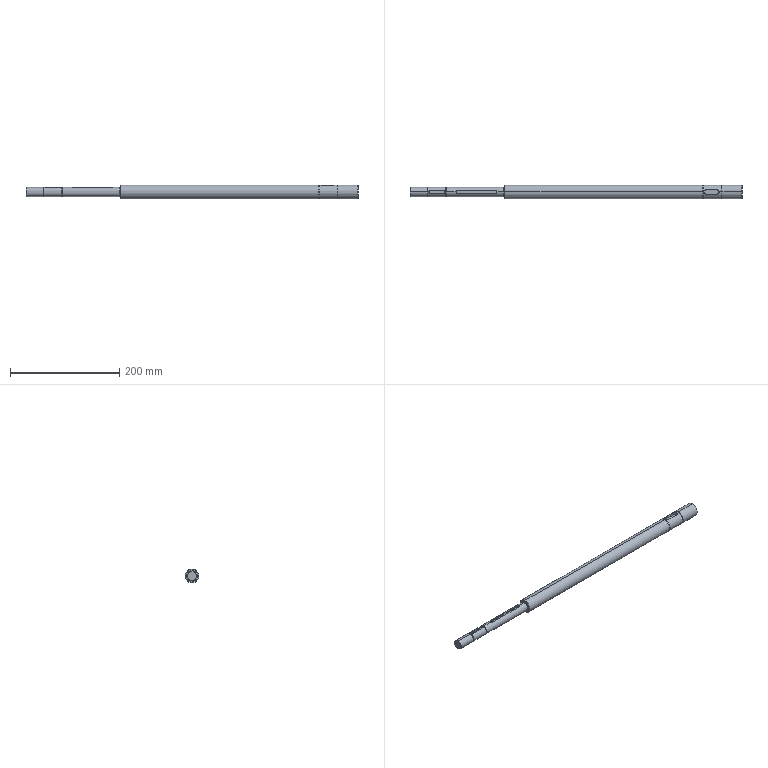Part | SolidWorks | features ICE 3, Chamfer 2, LPattern 2, RevCut 2, Extrusion 1, Fillet 1 | 1 solid | 57 faces | box 609 x 25 x 25 mm | volume 250736 mm3 | cylinder 29 | plane 20 | cone 6 | torus 2 | commonest cylinder face diameters 5 x6 17 x6 25 x6 16.2 x4 23.9 x4 8 x3